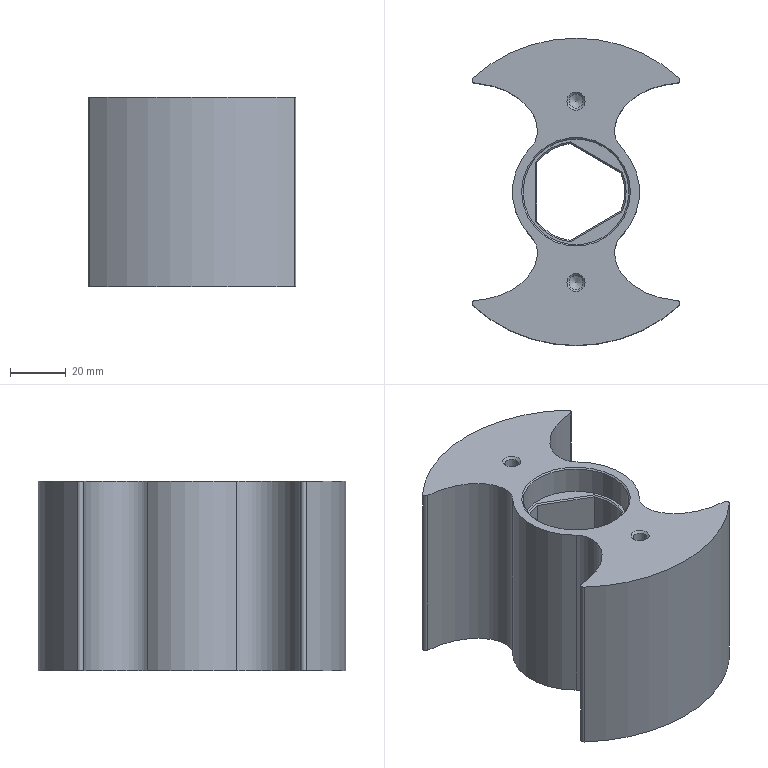CAM job | NX | 3-axis milling, drilling | part box 74.46 x 110.159 x 68 mm | stock box 110.159 x 110.159 x 68 mm
Tools:
number,name,description,diameter,corner_radius,flute_length,length,flutes
1,ZXZ,Milling Tool-5 Parameters,6.0,0.0,50.0,75.0,2
12,D12,Milling Tool-5 Parameters,12.0,0.0,50.0,75.0,2
5,D25R0.5,Milling Tool-5 Parameters,25.0,0.5,50.0,75.0,2
7,D6A45,Milling Tool-5 Parameters,6.0,0.0,50.0,75.0,2
12,2.5ZT,Drilling Tool,2.5,0.0,35.0,50.0,2
Operations:
program,operation,operation_type,tool,method,geometry_group,spindle_rpm,surface_speed,feed_per_tooth,feed_cut,feed_plunge,cut_length_mm,path_length_mm,cut_time_min,machine_time_min
1,DRILLING_COPY_1,Operation,ZXZ,METHOD,C,5000.0,94.0,0.025,250.0,0.0,8.0,119.611,0.032,0.0432
1,DRILLING_COPY_1_COPY,Operation,2.5ZT,METHOD,C,2000.0,15.0,0.03,120.0,0.0,21.502,146.615,0.1792,0.1917
1,ZLEVEL_PROFILE_COPY_1,ZLevelMilling,D12,METHOD,C,3000.0,113.0,0.3,1800.0,1000.0,17438.518,17555.318,9.742,9.754
1,刀补12_1,ZLevelMilling,D12,METHOD,C,5000.0,157.0,0.125,1250.0,100.0,4104.219,10561.748,3.283,3.929
2,ZLEVEL_PROFILE_COPY_2,ZLevelMilling,D25R0.5,METHOD,C,2000.0,157.0,0.55,2200.0,1000.0,58705.99,157478.922,28.135,38.012
2,ZLEVEL_PROFILE,ZLevelMilling,D25R0.5,METHOD,C,2000.0,157.0,0.55,2200.0,1000.0,55715.274,147806.668,26.175,35.384
2,刀补12,ZLevelMilling,D12,METHOD,C,5000.0,157.0,0.125,1250.0,100.0,18499.278,41320.734,14.799,17.082
2,PLANAR_MILL_COPY_COPY,PlanarMilling,D6A45,METHOD,C,7500.0,141.0,0.0833,1250.0,100.0,538.792,863.064,0.431,0.4635